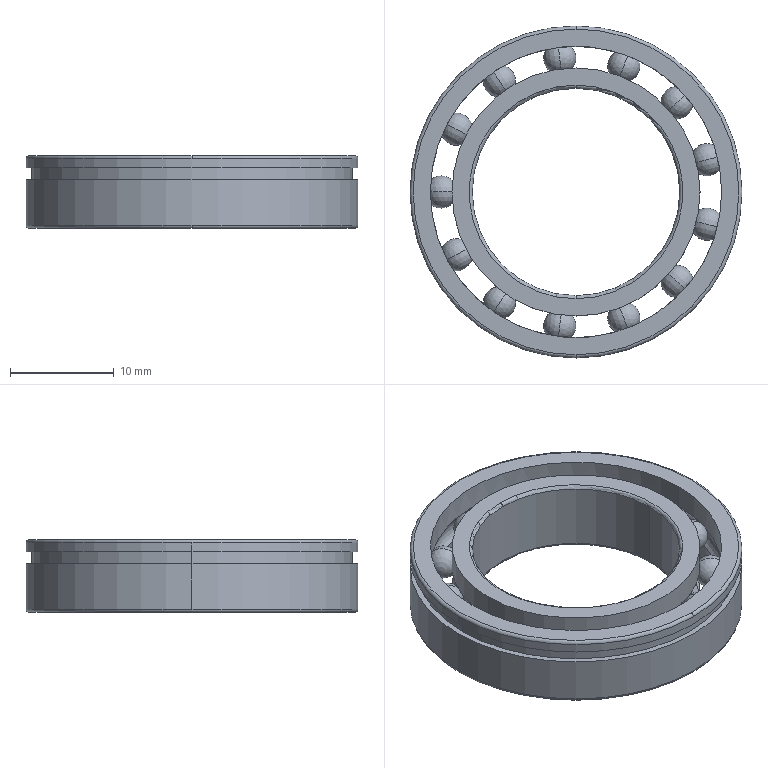Part | SolidWorks | 15 solids | 62 faces | box 32 x 32 x 7 mm | volume 2240 mm3 | sphere 26 | cylinder 16 | torus 14 | plane 6 | commonest cylinder face diameters 23.912 x4 28.088 x4 32 x4 20 x2 30.92 x2